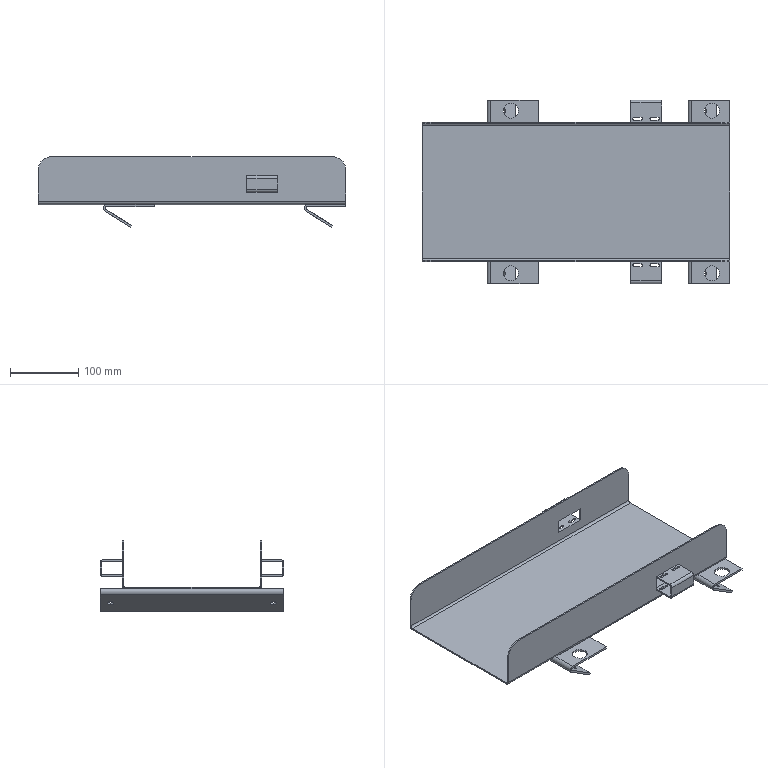Part | STEP file | NG chute S | 1 solid | 124 faces | box 450 x 268 x 103.148 mm | volume 495512 mm3 | plane 64 | cylinder 60 | commonest cylinder face diameters 4 x30 9 x8 22 x8 8 x4 10 x4 40 x4